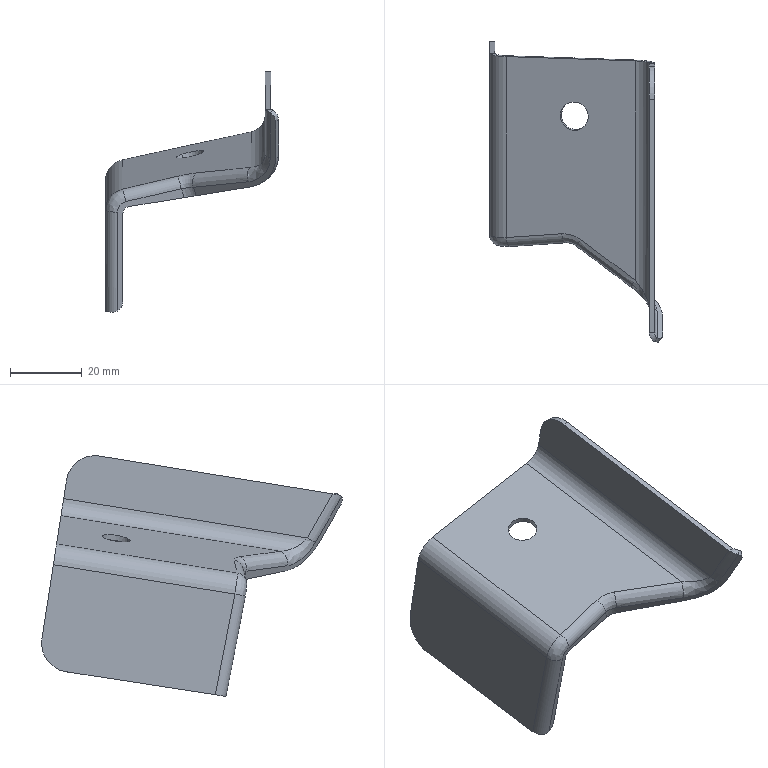Part | 1 solid | 54 faces | box 48.241 x 83.823 x 67.089 mm | volume 8502 mm3 | spline 34 | cylinder 11 | plane 9 | commonest cylinder face diameters 3 x2 6 x2 8 x2 9 x1 10 x1 12 x1